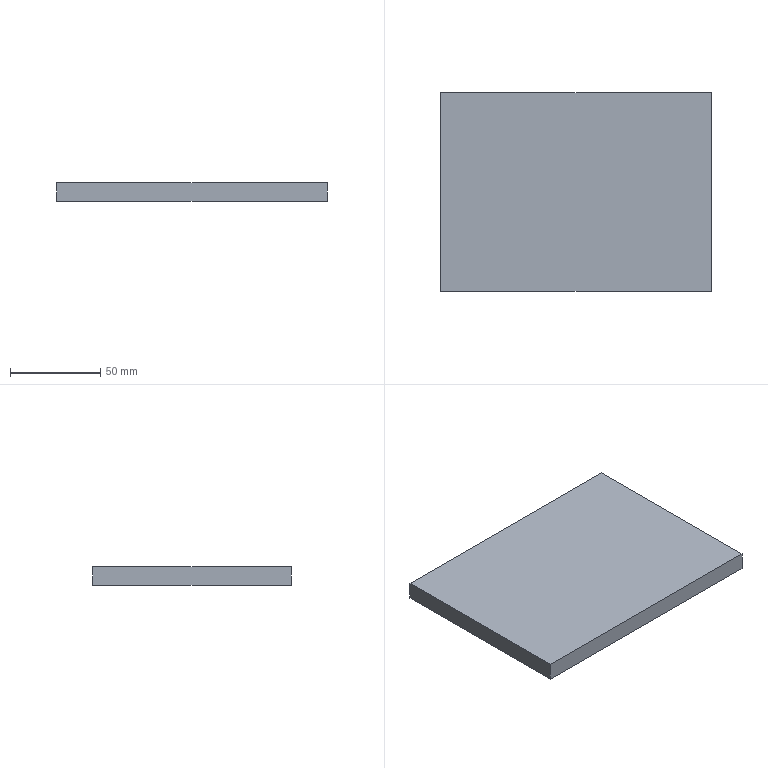Part | STEP file | MYT-A01-P18 | 1 solid | 6 faces | box 150 x 110 x 10 mm | volume 165000 mm3 | plane 6
STEP:
#1=CARTESIAN_POINT('',(75.,-55.,0.));
#2=VERTEX_POINT('',#1);
#3=CARTESIAN_POINT('',(75.,55.,0.));
#4=VERTEX_POINT('',#3);
#5=CARTESIAN_POINT('',(75.,55.,0.));
#6=DIRECTION('',(0.,1.,0.));
#7=VECTOR('',#6,1000.);
#8=LINE('',#5,#7);
#9=EDGE_CURVE('',#2,#4,#8,.T.);
#10=ORIENTED_EDGE('',*,*,#9,.T.);
#11=CARTESIAN_POINT('',(75.,55.,10.));
#12=VERTEX_POINT('',#11);
#13=CARTESIAN_POINT('',(75.,55.,10.));
#14=DIRECTION('',(0.,0.,-1.));
#15=VECTOR('',#14,1000.);
#16=LINE('',#13,#15);
#17=EDGE_CURVE('',#12,#4,#16,.T.);
#18=ORIENTED_EDGE('',*,*,#17,.F.);
#19=CARTESIAN_POINT('',(75.,-55.,10.));
#20=VERTEX_POINT('',#19);
#21=CARTESIAN_POINT('',(75.,55.,10.));
#22=DIRECTION('',(0.,1.,0.));
#23=VECTOR('',#22,1000.);
#24=LINE('',#21,#23);
#25=EDGE_CURVE('',#20,#12,#24,.T.);
#26=ORIENTED_EDGE('',*,*,#25,.F.);
#27=CARTESIAN_POINT('',(75.,-55.,10.));
#28=DIRECTION('',(0.,0.,-1.));
#29=VECTOR('',#28,1000.);
#30=LINE('',#27,#29);
#31=EDGE_CURVE('',#20,#2,#30,.T.);
#32=ORIENTED_EDGE('',*,*,#31,.T.);
#33=EDGE_LOOP('',(#10,#18,#26,#32));
#34=FACE_OUTER_BOUND('',#33,.T.);
#35=CARTESIAN_POINT('',(75.,55.,10.));
#36=DIRECTION('',(-1.,0.,0.));
#37=DIRECTION('',(0.,-1.,0.));
#38=AXIS2_PLACEMENT_3D('',#35,#36,#37);
#39=PLANE('',#38);
#40=ADVANCED_FACE('',(#34),#39,.F.);
#41=CARTESIAN_POINT('',(-75.,55.,0.));
#42=VERTEX_POINT('',#41);
#43=CARTESIAN_POINT('',(-75.,55.,0.));
#44=DIRECTION('',(-1.,0.,0.));
#45=VECTOR('',#44,1000.);
#46=LINE('',#43,#45);
#47=EDGE_CURVE('',#4,#42,#46,.T.);
#48=ORIENTED_EDGE('',*,*,#47,.T.);
#49=CARTESIAN_POINT('',(-75.,55.,10.));
#50=VERTEX_POINT('',#49);
#51=CARTESIAN_POINT('',(-75.,55.,10.));
#52=DIRECTION('',(0.,0.,-1.));
#53=VECTOR('',#52,1000.);
#54=LINE('',#51,#53);
#55=EDGE_CURVE('',#50,#42,#54,.T.);
#56=ORIENTED_EDGE('',*,*,#55,.F.);
#57=CARTESIAN_POINT('',(-75.,55.,10.));
#58=DIRECTION('',(-1.,0.,0.));
#59=VECTOR('',#58,1000.);
#60=LINE('',#57,#59);
#61=EDGE_CURVE('',#12,#50,#60,.T.);
#62=ORIENTED_EDGE('',*,*,#61,.F.);
#63=ORIENTED_EDGE('',*,*,#17,.T.);
#64=EDGE_LOOP('',(#48,#56,#62,#63));
#65=FACE_OUTER_BOUND('',#64,.T.);
#66=CARTESIAN_POINT('',(-75.,55.,10.));
#67=DIRECTION('',(0.,-1.,0.));
#68=DIRECTION('',(0.,0.,-1.));
#69=AXIS2_PLACEMENT_3D('',#66,#67,#68);
#70=PLANE('',#69);
#71=ADVANCED_FACE('',(#65),#70,.F.);
#72=CARTESIAN_POINT('',(-75.,-55.,0.));
#73=VERTEX_POINT('',#72);
#74=CARTESIAN_POINT('',(-75.,55.,0.));
#75=DIRECTION('',(0.,-1.,0.));
#76=VECTOR('',#75,1000.);
#77=LINE('',#74,#76);
#78=EDGE_CURVE('',#42,#73,#77,.T.);
#79=ORIENTED_EDGE('',*,*,#78,.T.);
#80=CARTESIAN_POINT('',(-75.,-55.,10.));
#81=VERTEX_POINT('',#80);
#82=CARTESIAN_POINT('',(-75.,-55.,10.));
#83=DIRECTION('',(0.,0.,-1.));
#84=VECTOR('',#83,1000.);
#85=LINE('',#82,#84);
#86=EDGE_CURVE('',#81,#73,#85,.T.);
#87=ORIENTED_EDGE('',*,*,#86,.F.);
#88=CARTESIAN_POINT('',(-75.,55.,10.));
#89=DIRECTION('',(0.,-1.,0.));
#90=VECTOR('',#89,1000.);
#91=LINE('',#88,#90);
#92=EDGE_CURVE('',#50,#81,#91,.T.);
#93=ORIENTED_EDGE('',*,*,#92,.F.);
#94=ORIENTED_EDGE('',*,*,#55,.T.);
#95=EDGE_LOOP('',(#79,#87,#93,#94));
#96=FACE_OUTER_BOUND('',#95,.T.);
#97=CARTESIAN_POINT('',(-75.,55.,10.));
#98=DIRECTION('',(1.,0.,0.));
#99=DIRECTION('',(0.,1.,0.));
#100=AXIS2_PLACEMENT_3D('',#97,#98,#99);
#101=PLANE('',#100);
#102=ADVANCED_FACE('',(#96),#101,.F.);
#103=CARTESIAN_POINT('',(-75.,-55.,0.));
#104=DIRECTION('',(1.,0.,0.));
#105=VECTOR('',#104,1000.);
#106=LINE('',#103,#105);
#107=EDGE_CURVE('',#73,#2,#106,.T.);
#108=ORIENTED_EDGE('',*,*,#107,.T.);
#109=ORIENTED_EDGE('',*,*,#31,.F.);
#110=CARTESIAN_POINT('',(-75.,-55.,10.));
#111=DIRECTION('',(1.,0.,0.));
#112=VECTOR('',#111,1000.);
#113=LINE('',#110,#112);
#114=EDGE_CURVE('',#81,#20,#113,.T.);
#115=ORIENTED_EDGE('',*,*,#114,.F.);
#116=ORIENTED_EDGE('',*,*,#86,.T.);
#117=EDGE_LOOP('',(#108,#109,#115,#116));
#118=FACE_OUTER_BOUND('',#117,.T.);
#119=CARTESIAN_POINT('',(-75.,-55.,10.));
#120=DIRECTION('',(0.,1.,0.));
#121=DIRECTION('',(0.,0.,1.));
#122=AXIS2_PLACEMENT_3D('',#119,#120,#121);
#123=PLANE('',#122);
#124=ADVANCED_FACE('',(#118),#123,.F.);
#125=ORIENTED_EDGE('',*,*,#25,.T.);
#126=ORIENTED_EDGE('',*,*,#61,.T.);
#127=ORIENTED_EDGE('',*,*,#92,.T.);
#128=ORIENTED_EDGE('',*,*,#114,.T.);
#129=EDGE_LOOP('',(#125,#126,#127,#128));
#130=FACE_OUTER_BOUND('',#129,.T.);
#131=CARTESIAN_POINT('',(0.,0.,10.));
#132=DIRECTION('',(0.,0.,1.));
#133=DIRECTION('',(1.,0.,0.));
#134=AXIS2_PLACEMENT_3D('',#131,#132,#133);
#135=PLANE('',#134);
#136=ADVANCED_FACE('',(#130),#135,.T.);
#137=ORIENTED_EDGE('',*,*,#9,.F.);
#138=ORIENTED_EDGE('',*,*,#107,.F.);
#139=ORIENTED_EDGE('',*,*,#78,.F.);
#140=ORIENTED_EDGE('',*,*,#47,.F.);
#141=EDGE_LOOP('',(#137,#138,#139,#140));
#142=FACE_OUTER_BOUND('',#141,.T.);
#143=CARTESIAN_POINT('',(0.,0.,0.));
#144=DIRECTION('',(0.,0.,1.));
#145=DIRECTION('',(1.,0.,0.));
#146=AXIS2_PLACEMENT_3D('',#143,#144,#145);
#147=PLANE('',#146);
#148=ADVANCED_FACE('',(#142),#147,.F.);
#149=CLOSED_SHELL('',(#40,#71,#102,#124,#136,#148));
#150=MANIFOLD_SOLID_BREP('',#149);
#151=CARTESIAN_POINT('',(0.,0.,0.));
#152=DIRECTION('',(0.,0.,1.));
#153=DIRECTION('',(1.,0.,0.));
#154=AXIS2_PLACEMENT_3D('',#151,#152,#153);
#155=(LENGTH_UNIT()NAMED_UNIT(*)SI_UNIT(.MILLI.,.METRE.));
#156=UNCERTAINTY_MEASURE_WITH_UNIT(LENGTH_MEASURE(0.00001),#155,'','');
#157=(NAMED_UNIT(*)PLANE_ANGLE_UNIT()SI_UNIT($,.RADIAN.));
#158=(NAMED_UNIT(*)SI_UNIT($,.STERADIAN.)SOLID_ANGLE_UNIT());
#159=(GEOMETRIC_REPRESENTATION_CONTEXT(3)GLOBAL_UNCERTAINTY_ASSIGNED_CONTEXT((#156))GLOBAL_UNIT_ASSIGNED_CONTEXT((#155,#157,#158))REPRESENTATION_CONTEXT('',''));
#160=ADVANCED_BREP_SHAPE_REPRESENTATION('',(#150,#154),#159);